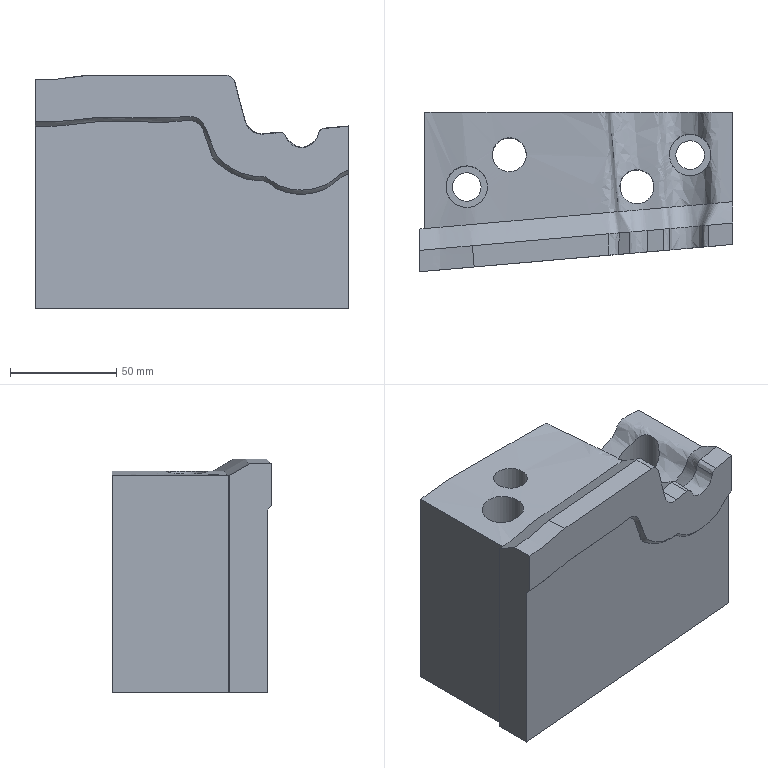Part | NX | features solid 2 | 1 solid | 29 faces | box 147.3 x 75 x 110.018 mm | volume 845092 mm3 | spline 13 | plane 10 | cylinder 6 | commonest cylinder face diameters 13.5 x2 16 x2 19.5 x2